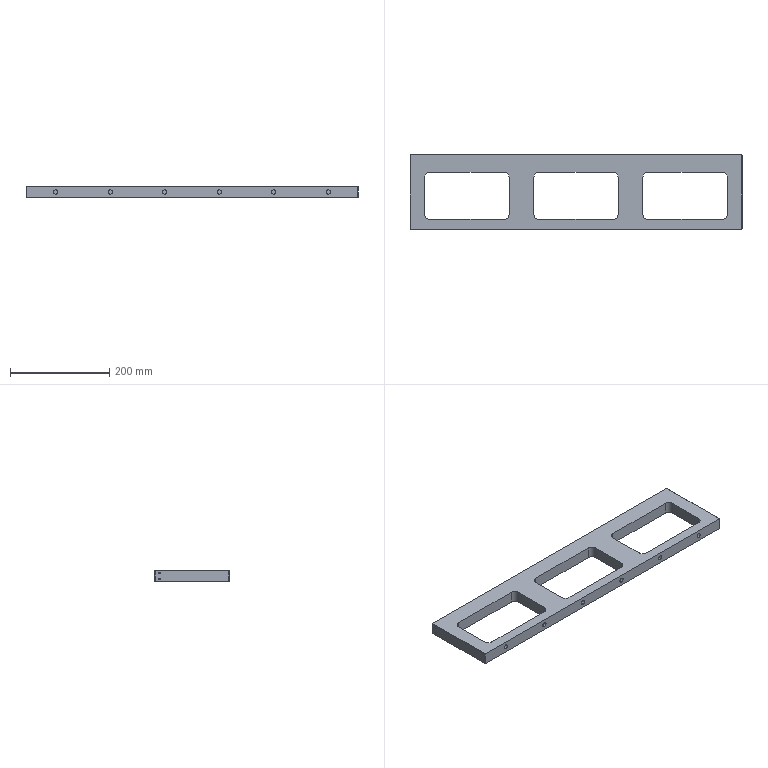Part | SolidWorks | features HoleWzd 7, Chamfer 1, Extrusion 1, ICE 1 | 1 solid | 146 faces | box 670 x 150 x 24 mm | volume 1244825 mm3 | cylinder 72 | cone 48 | plane 26 | commonest cylinder face diameters 3.3 x34 9 x12 20 x12 2.5 x8 6 x6